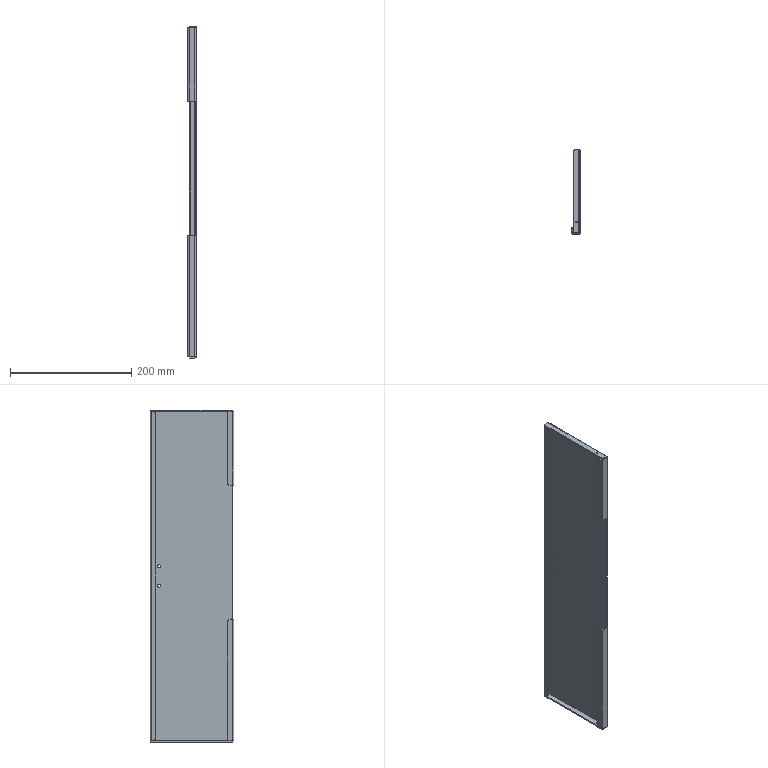Part | STEP file | keyboard and mouse push plate | 1 solid | 98 faces | box 14 x 138 x 548 mm | volume 182409 mm3 | plane 60 | cylinder 34 | spline 4 | commonest cylinder face diameters 4 x10 0.2 x8 4.2 x8 2.5 x4 5 x4